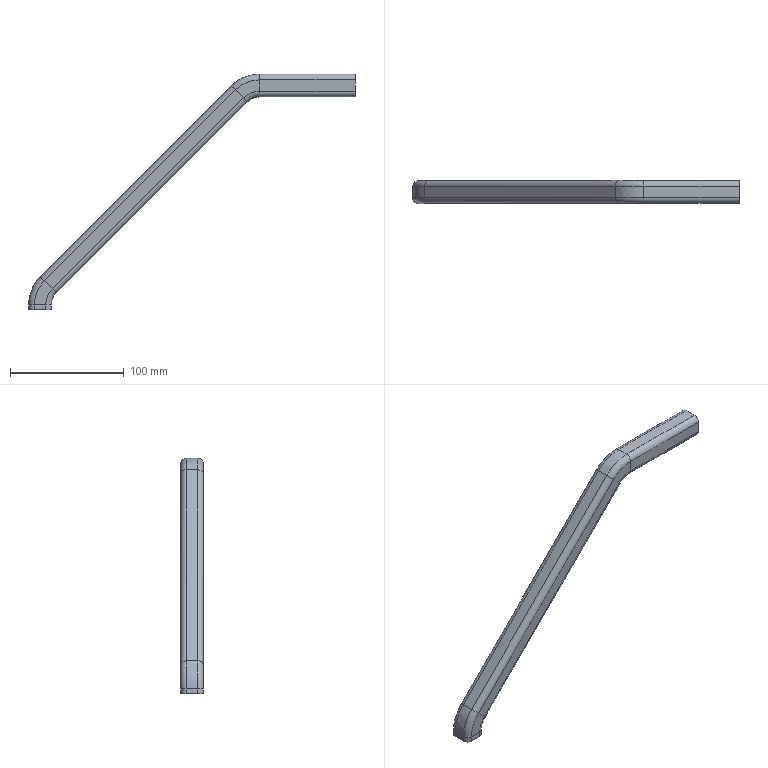Part | NX | features BREP 1 | 1 solid | 104 faces | box 286.954 x 20 x 207.051 mm | volume 47543 mm3 | plane 48 | cylinder 40 | torus 16 | commonest cylinder face diameters 6 x16 10.001 x8 10 x4 34 x4 66 x4 30 x2